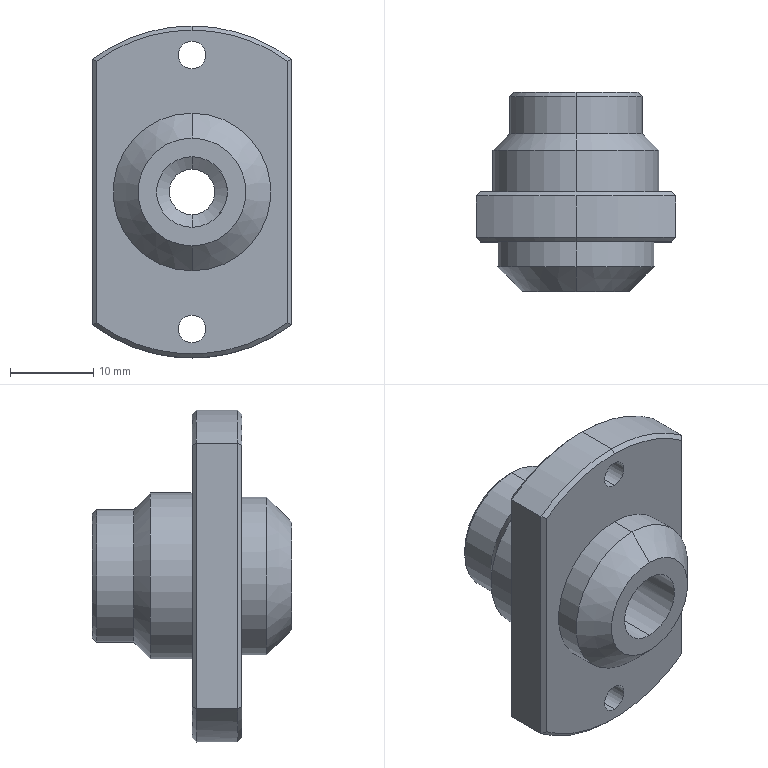Part | SolidWorks | features ICE 7, Chamfer 4, HoleWzd 4, Extrusion 1, RevCut 1 | 1 solid | 52 faces | box 24 x 24 x 40 mm | volume 8141 mm3 | cylinder 25 | cone 14 | plane 13 | commonest cylinder face diameters 3.3 x4 11 x4 40 x3 4.2 x2 5.5 x2 8.5 x2
STEP:
#1=CARTESIAN_POINT('',(0.,-5.,8.));
#2=VERTEX_POINT('',#1);
#3=CARTESIAN_POINT('',(0.,-5.,-8.));
#4=VERTEX_POINT('',#3);
#5=CARTESIAN_POINT('',(0.,-5.,0.));
#6=DIRECTION('',(0.,1.,0.));
#7=DIRECTION('',(0.,0.,1.));
#8=AXIS2_PLACEMENT_3D('',#5,#6,#7);
#9=CIRCLE('',#8,8.);
#10=EDGE_CURVE('',#2,#4,#9,.T.);
#11=ORIENTED_EDGE('',*,*,#10,.F.);
#12=CARTESIAN_POINT('',(0.,-7.,10.));
#13=VERTEX_POINT('',#12);
#14=CARTESIAN_POINT('',(0.,-7.,10.));
#15=DIRECTION('',(0.,-0.7071,0.7071));
#16=VECTOR('',#15,1000.);
#17=LINE('',#14,#16);
#18=EDGE_CURVE('',#2,#13,#17,.T.);
#19=ORIENTED_EDGE('',*,*,#18,.T.);
#20=CARTESIAN_POINT('',(0.,-7.,-10.));
#21=VERTEX_POINT('',#20);
#22=CARTESIAN_POINT('',(0.,-7.,0.));
#23=DIRECTION('',(0.,1.,0.));
#24=DIRECTION('',(0.,0.,1.));
#25=AXIS2_PLACEMENT_3D('',#22,#23,#24);
#26=CIRCLE('',#25,10.);
#27=EDGE_CURVE('',#13,#21,#26,.T.);
#28=ORIENTED_EDGE('',*,*,#27,.T.);
#29=CARTESIAN_POINT('',(0.,-7.,-10.));
#30=DIRECTION('',(0.,-0.7071,-0.7071));
#31=VECTOR('',#30,1000.);
#32=LINE('',#29,#31);
#33=EDGE_CURVE('',#4,#21,#32,.T.);
#34=ORIENTED_EDGE('',*,*,#33,.F.);
#35=EDGE_LOOP('',(#11,#19,#28,#34));
#36=FACE_OUTER_BOUND('',#35,.T.);
#37=CARTESIAN_POINT('',(0.,-7.,0.));
#38=DIRECTION('',(0.,-1.,0.));
#39=DIRECTION('',(0.,0.,-1.));
#40=AXIS2_PLACEMENT_3D('',#37,#38,#39);
#41=CONICAL_SURFACE('',#40,10.,0.7854);
#42=ADVANCED_FACE('',(#36),#41,.T.);
#43=ORIENTED_EDGE('',*,*,#27,.F.);
#44=CARTESIAN_POINT('',(0.,-12.,10.));
#45=VERTEX_POINT('',#44);
#46=CARTESIAN_POINT('',(0.,-7.,10.));
#47=DIRECTION('',(0.,-1.,0.));
#48=VECTOR('',#47,1000.);
#49=LINE('',#46,#48);
#50=EDGE_CURVE('',#13,#45,#49,.T.);
#51=ORIENTED_EDGE('',*,*,#50,.T.);
#52=CARTESIAN_POINT('',(0.,-12.,-10.));
#53=VERTEX_POINT('',#52);
#54=CARTESIAN_POINT('',(0.,-12.,0.));
#55=DIRECTION('',(0.,1.,0.));
#56=DIRECTION('',(0.,0.,-1.));
#57=AXIS2_PLACEMENT_3D('',#54,#55,#56);
#58=CIRCLE('',#57,10.);
#59=EDGE_CURVE('',#45,#53,#58,.T.);
#60=ORIENTED_EDGE('',*,*,#59,.T.);
#61=CARTESIAN_POINT('',(0.,-7.,-10.));
#62=DIRECTION('',(0.,-1.,0.));
#63=VECTOR('',#62,1000.);
#64=LINE('',#61,#63);
#65=EDGE_CURVE('',#21,#53,#64,.T.);
#66=ORIENTED_EDGE('',*,*,#65,.F.);
#67=EDGE_LOOP('',(#43,#51,#60,#66));
#68=FACE_OUTER_BOUND('',#67,.T.);
#69=CARTESIAN_POINT('',(0.,-7.,0.));
#70=DIRECTION('',(0.,-1.,0.));
#71=DIRECTION('',(0.,0.,-1.));
#72=AXIS2_PLACEMENT_3D('',#69,#70,#71);
#73=CYLINDRICAL_SURFACE('',#72,10.);
#74=ADVANCED_FACE('',(#68),#73,.T.);
#75=CARTESIAN_POINT('',(0.,-2.,5.75));
#76=VERTEX_POINT('',#75);
#77=CARTESIAN_POINT('',(0.,-2.,-5.75));
#78=VERTEX_POINT('',#77);
#79=CARTESIAN_POINT('',(0.,-2.,0.));
#80=DIRECTION('',(0.,-1.,0.));
#81=DIRECTION('',(0.,0.,-1.));
#82=AXIS2_PLACEMENT_3D('',#79,#80,#81);
#83=CIRCLE('',#82,5.75);
#84=EDGE_CURVE('',#76,#78,#83,.T.);
#85=ORIENTED_EDGE('',*,*,#84,.F.);
#86=CARTESIAN_POINT('',(0.,-3.,5.75));
#87=VERTEX_POINT('',#86);
#88=CARTESIAN_POINT('',(0.,-12.,5.75));
#89=DIRECTION('',(0.,-1.,0.));
#90=VECTOR('',#89,1000.);
#91=LINE('',#88,#90);
#92=EDGE_CURVE('',#76,#87,#91,.T.);
#93=ORIENTED_EDGE('',*,*,#92,.T.);
#94=CARTESIAN_POINT('',(0.,-3.,-5.75));
#95=VERTEX_POINT('',#94);
#96=CARTESIAN_POINT('',(0.,-3.,0.));
#97=DIRECTION('',(0.,-1.,0.));
#98=DIRECTION('',(0.,0.,-1.));
#99=AXIS2_PLACEMENT_3D('',#96,#97,#98);
#100=CIRCLE('',#99,5.75);
#101=EDGE_CURVE('',#87,#95,#100,.T.);
#102=ORIENTED_EDGE('',*,*,#101,.T.);
#103=CARTESIAN_POINT('',(0.,-12.,-5.75));
#104=DIRECTION('',(0.,-1.,0.));
#105=VECTOR('',#104,1000.);
#106=LINE('',#103,#105);
#107=EDGE_CURVE('',#78,#95,#106,.T.);
#108=ORIENTED_EDGE('',*,*,#107,.F.);
#109=EDGE_LOOP('',(#85,#93,#102,#108));
#110=FACE_OUTER_BOUND('',#109,.T.);
#111=CARTESIAN_POINT('',(0.,-12.,0.));
#112=DIRECTION('',(0.,-1.,0.));
#113=DIRECTION('',(0.,0.,-1.));
#114=AXIS2_PLACEMENT_3D('',#111,#112,#113);
#115=CYLINDRICAL_SURFACE('',#114,5.75);
#116=ADVANCED_FACE('',(#110),#115,.F.);
#117=CARTESIAN_POINT('',(0.,0.,7.5));
#118=VERTEX_POINT('',#117);
#119=CARTESIAN_POINT('',(0.,0.,-7.5));
#120=VERTEX_POINT('',#119);
#121=CARTESIAN_POINT('',(0.,0.,0.));
#122=DIRECTION('',(0.,1.,0.));
#123=DIRECTION('',(0.,0.,1.));
#124=AXIS2_PLACEMENT_3D('',#121,#122,#123);
#125=CIRCLE('',#124,7.5);
#126=EDGE_CURVE('',#118,#120,#125,.T.);
#127=ORIENTED_EDGE('',*,*,#126,.F.);
#128=CARTESIAN_POINT('',(0.,-0.5,8.));
#129=VERTEX_POINT('',#128);
#130=CARTESIAN_POINT('',(0.,0.,7.5));
#131=DIRECTION('',(0.,-0.7071,0.7071));
#132=VECTOR('',#131,1000.);
#133=LINE('',#130,#132);
#134=EDGE_CURVE('',#118,#129,#133,.T.);
#135=ORIENTED_EDGE('',*,*,#134,.T.);
#136=CARTESIAN_POINT('',(0.,-0.5,-8.));
#137=VERTEX_POINT('',#136);
#138=CARTESIAN_POINT('',(0.,-0.5,0.));
#139=DIRECTION('',(0.,-1.,0.));
#140=DIRECTION('',(0.,0.,1.));
#141=AXIS2_PLACEMENT_3D('',#138,#139,#140);
#142=CIRCLE('',#141,8.);
#143=EDGE_CURVE('',#137,#129,#142,.T.);
#144=ORIENTED_EDGE('',*,*,#143,.F.);
#145=CARTESIAN_POINT('',(0.,0.,-7.5));
#146=DIRECTION('',(0.,-0.7071,-0.7071));
#147=VECTOR('',#146,1000.);
#148=LINE('',#145,#147);
#149=EDGE_CURVE('',#120,#137,#148,.T.);
#150=ORIENTED_EDGE('',*,*,#149,.F.);
#151=EDGE_LOOP('',(#127,#135,#144,#150));
#152=FACE_OUTER_BOUND('',#151,.T.);
#153=CARTESIAN_POINT('',(0.,0.,0.));
#154=DIRECTION('',(0.,-1.,0.));
#155=DIRECTION('',(0.,0.,-1.));
#156=AXIS2_PLACEMENT_3D('',#153,#154,#155);
#157=CONICAL_SURFACE('',#156,7.5,0.7854);
#158=ADVANCED_FACE('',(#152),#157,.T.);
#159=CARTESIAN_POINT('',(0.,-12.,-19.5));
#160=VERTEX_POINT('',#159);
#161=CARTESIAN_POINT('',(-11.5,-12.,-15.748));
#162=VERTEX_POINT('',#161);
#163=CARTESIAN_POINT('',(0.,-12.,0.));
#164=DIRECTION('',(0.,1.,0.));
#165=DIRECTION('',(0.,0.,-1.));
#166=AXIS2_PLACEMENT_3D('',#163,#164,#165);
#167=CIRCLE('',#166,19.5);
#168=EDGE_CURVE('',#160,#162,#167,.T.);
#169=ORIENTED_EDGE('',*,*,#168,.F.);
#170=CARTESIAN_POINT('',(0.,-12.5,-20.));
#171=VERTEX_POINT('',#170);
#172=CARTESIAN_POINT('',(0.,-12.5,-20.));
#173=DIRECTION('',(0.,-0.7071,-0.7071));
#174=VECTOR('',#173,1000.);
#175=LINE('',#172,#174);
#176=EDGE_CURVE('',#160,#171,#175,.T.);
#177=ORIENTED_EDGE('',*,*,#176,.T.);
#178=CARTESIAN_POINT('',(-12.,-12.5,-16.));
#179=VERTEX_POINT('',#178);
#180=CARTESIAN_POINT('',(0.,-12.5,0.));
#181=DIRECTION('',(0.,-1.,0.));
#182=DIRECTION('',(0.,0.,-1.));
#183=AXIS2_PLACEMENT_3D('',#180,#181,#182);
#184=CIRCLE('',#183,20.);
#185=EDGE_CURVE('',#179,#171,#184,.T.);
#186=ORIENTED_EDGE('',*,*,#185,.F.);
#187=CARTESIAN_POINT('',(-11.5,-12.,-15.748));
#188=CARTESIAN_POINT('',(-11.667,-12.167,-15.833));
#189=CARTESIAN_POINT('',(-11.833,-12.333,-15.917));
#190=CARTESIAN_POINT('',(-12.,-12.5,-16.));
#191=B_SPLINE_CURVE_WITH_KNOTS('',3,(#187,#188,#189,#190),.UNSPECIFIED.,.F.,.F.,(4,4),(0.,0.0007507),.UNSPECIFIED.);
#192=EDGE_CURVE('',#162,#179,#191,.T.);
#193=ORIENTED_EDGE('',*,*,#192,.F.);
#194=EDGE_LOOP('',(#169,#177,#186,#193));
#195=FACE_OUTER_BOUND('',#194,.T.);
#196=CARTESIAN_POINT('',(0.,-12.5,0.));
#197=DIRECTION('',(0.,-1.,0.));
#198=DIRECTION('',(0.,0.,-1.));
#199=AXIS2_PLACEMENT_3D('',#196,#197,#198);
#200=CONICAL_SURFACE('',#199,20.,0.7854);
#201=ADVANCED_FACE('',(#195),#200,.T.);
#202=CARTESIAN_POINT('',(0.,-18.,19.5));
#203=VERTEX_POINT('',#202);
#204=CARTESIAN_POINT('',(-11.5,-18.,15.748));
#205=VERTEX_POINT('',#204);
#206=CARTESIAN_POINT('',(0.,-18.,0.));
#207=DIRECTION('',(0.,-1.,0.));
#208=DIRECTION('',(0.,0.,-1.));
#209=AXIS2_PLACEMENT_3D('',#206,#207,#208);
#210=CIRCLE('',#209,19.5);
#211=EDGE_CURVE('',#203,#205,#210,.T.);
#212=ORIENTED_EDGE('',*,*,#211,.F.);
#213=CARTESIAN_POINT('',(0.,-17.5,20.));
#214=VERTEX_POINT('',#213);
#215=CARTESIAN_POINT('',(0.,-18.,19.5));
#216=DIRECTION('',(0.,0.7071,0.7071));
#217=VECTOR('',#216,1000.);
#218=LINE('',#215,#217);
#219=EDGE_CURVE('',#203,#214,#218,.T.);
#220=ORIENTED_EDGE('',*,*,#219,.T.);
#221=CARTESIAN_POINT('',(-12.,-17.5,16.));
#222=VERTEX_POINT('',#221);
#223=CARTESIAN_POINT('',(0.,-17.5,0.));
#224=DIRECTION('',(0.,1.,0.));
#225=DIRECTION('',(0.,0.,-1.));
#226=AXIS2_PLACEMENT_3D('',#223,#224,#225);
#227=CIRCLE('',#226,20.);
#228=EDGE_CURVE('',#222,#214,#227,.T.);
#229=ORIENTED_EDGE('',*,*,#228,.F.);
#230=CARTESIAN_POINT('',(-11.5,-18.,15.748));
#231=CARTESIAN_POINT('',(-11.667,-17.833,15.833));
#232=CARTESIAN_POINT('',(-11.833,-17.667,15.917));
#233=CARTESIAN_POINT('',(-12.,-17.5,16.));
#234=B_SPLINE_CURVE_WITH_KNOTS('',3,(#230,#231,#232,#233),.UNSPECIFIED.,.F.,.F.,(4,4),(0.,0.0007507),.UNSPECIFIED.);
#235=EDGE_CURVE('',#205,#222,#234,.T.);
#236=ORIENTED_EDGE('',*,*,#235,.F.);
#237=EDGE_LOOP('',(#212,#220,#229,#236));
#238=FACE_OUTER_BOUND('',#237,.T.);
#239=CARTESIAN_POINT('',(0.,-18.,0.));
#240=DIRECTION('',(0.,1.,0.));
#241=DIRECTION('',(0.,0.,1.));
#242=AXIS2_PLACEMENT_3D('',#239,#240,#241);
#243=CONICAL_SURFACE('',#242,19.5,0.7854);
#244=ADVANCED_FACE('',(#238),#243,.T.);
#245=CARTESIAN_POINT('',(3.695,-15.,2.1));
#246=VERTEX_POINT('',#245);
#247=CARTESIAN_POINT('',(3.695,-15.,-2.1));
#248=VERTEX_POINT('',#247);
#249=CARTESIAN_POINT('',(3.695,-15.,2.1));
#250=CARTESIAN_POINT('',(3.695,-15.139,2.1));
#251=CARTESIAN_POINT('',(3.703,-15.281,2.086));
#252=CARTESIAN_POINT('',(3.734,-15.552,2.031));
#253=CARTESIAN_POINT('',(3.756,-15.684,1.99));
#254=CARTESIAN_POINT('',(3.81,-15.939,1.883));
#255=CARTESIAN_POINT('',(3.842,-16.059,1.819));
#256=CARTESIAN_POINT('',(3.91,-16.284,1.668));
#257=CARTESIAN_POINT('',(3.947,-16.389,1.58));
#258=CARTESIAN_POINT('',(4.018,-16.58,1.39));
#259=CARTESIAN_POINT('',(4.053,-16.666,1.286));
#260=CARTESIAN_POINT('',(4.117,-16.818,1.06));
#261=CARTESIAN_POINT('',(4.147,-16.884,0.938));
#262=CARTESIAN_POINT('',(4.196,-16.99,0.686));
#263=CARTESIAN_POINT('',(4.216,-17.03,0.5547));
#264=CARTESIAN_POINT('',(4.243,-17.086,0.2804));
#265=CARTESIAN_POINT('',(4.25,-17.1,0.1406));
#266=CARTESIAN_POINT('',(4.25,-17.1,-0.1373));
#267=CARTESIAN_POINT('',(4.243,-17.086,-0.2781));
#268=CARTESIAN_POINT('',(4.216,-17.031,-0.5516));
#269=CARTESIAN_POINT('',(4.197,-16.99,-0.6835));
#270=CARTESIAN_POINT('',(4.123,-16.831,-1.065));
#271=CARTESIAN_POINT('',(4.053,-16.676,-1.294));
#272=CARTESIAN_POINT('',(3.946,-16.388,-1.582));
#273=CARTESIAN_POINT('',(3.91,-16.284,-1.667));
#274=CARTESIAN_POINT('',(3.842,-16.059,-1.818));
#275=CARTESIAN_POINT('',(3.81,-15.938,-1.884));
#276=CARTESIAN_POINT('',(3.756,-15.685,-1.99));
#277=CARTESIAN_POINT('',(3.734,-15.555,-2.03));
#278=CARTESIAN_POINT('',(3.703,-15.283,-2.085));
#279=CARTESIAN_POINT('',(3.695,-15.141,-2.1));
#280=CARTESIAN_POINT('',(3.695,-15.,-2.1));
#281=B_SPLINE_CURVE_WITH_KNOTS('',3,(#249,#250,#251,#252,#253,#254,#255,#256,#257,#258,#259,#260,#261,#262,#263,#264,#265,#266,#267,#268,#269,#270,#271,#272,#273,#274,#275,#276,#277,#278,#279,#280),.UNSPECIFIED.,.F.,.F.,(4,2,2,2,2,2,2,2,2,2,2,2,2,2,2,4),(0.006676,0.007093,0.007509,0.007926,0.008343,0.008759,0.009176,0.009592,0.01001,0.01043,0.01084,0.01168,0.01209,0.01251,0.01292,0.01334),.UNSPECIFIED.);
#282=EDGE_CURVE('',#246,#248,#281,.T.);
#283=ORIENTED_EDGE('',*,*,#282,.F.);
#284=CARTESIAN_POINT('',(12.,-15.,2.1));
#285=VERTEX_POINT('',#284);
#286=CARTESIAN_POINT('',(12.,-15.,2.1));
#287=DIRECTION('',(1.,0.,0.));
#288=VECTOR('',#287,1000.);
#289=LINE('',#286,#288);
#290=EDGE_CURVE('',#246,#285,#289,.T.);
#291=ORIENTED_EDGE('',*,*,#290,.T.);
#292=CARTESIAN_POINT('',(12.,-15.,-2.1));
#293=VERTEX_POINT('',#292);
#294=CARTESIAN_POINT('',(12.,-15.,0.));
#295=DIRECTION('',(1.,0.,0.));
#296=DIRECTION('',(0.,0.,-1.));
#297=AXIS2_PLACEMENT_3D('',#294,#295,#296);
#298=CIRCLE('',#297,2.1);
#299=EDGE_CURVE('',#285,#293,#298,.T.);
#300=ORIENTED_EDGE('',*,*,#299,.T.);
#301=CARTESIAN_POINT('',(12.,-15.,-2.1));
#302=DIRECTION('',(1.,0.,0.));
#303=VECTOR('',#302,1000.);
#304=LINE('',#301,#303);
#305=EDGE_CURVE('',#248,#293,#304,.T.);
#306=ORIENTED_EDGE('',*,*,#305,.F.);
#307=EDGE_LOOP('',(#283,#291,#300,#306));
#308=FACE_OUTER_BOUND('',#307,.T.);
#309=CARTESIAN_POINT('',(12.,-15.,0.));
#310=DIRECTION('',(1.,0.,0.));
#311=DIRECTION('',(0.,0.,-1.));
#312=AXIS2_PLACEMENT_3D('',#309,#310,#311);
#313=CYLINDRICAL_SURFACE('',#312,2.1);
#314=ADVANCED_FACE('',(#308),#313,.F.);
#315=CARTESIAN_POINT('',(0.,-10.,4.25));
#316=VERTEX_POINT('',#315);
#317=CARTESIAN_POINT('',(0.,-10.,-4.25));
#318=VERTEX_POINT('',#317);
#319=CARTESIAN_POINT('',(0.,-10.,0.));
#320=DIRECTION('',(0.,-1.,0.));
#321=DIRECTION('',(0.,0.,-1.));
#322=AXIS2_PLACEMENT_3D('',#319,#320,#321);
#323=CIRCLE('',#322,4.25);
#324=EDGE_CURVE('',#316,#318,#323,.T.);
#325=ORIENTED_EDGE('',*,*,#324,.F.);
#326=CARTESIAN_POINT('',(0.,-24.,4.25));
#327=VERTEX_POINT('',#326);
#328=CARTESIAN_POINT('',(0.,-24.,4.25));
#329=DIRECTION('',(0.,-1.,0.));
#330=VECTOR('',#329,1000.);
#331=LINE('',#328,#330);
#332=EDGE_CURVE('',#316,#327,#331,.T.);
#333=ORIENTED_EDGE('',*,*,#332,.T.);
#334=CARTESIAN_POINT('',(0.,-24.,-4.25));
#335=VERTEX_POINT('',#334);
#336=CARTESIAN_POINT('',(0.,-24.,0.));
#337=DIRECTION('',(0.,-1.,0.));
#338=DIRECTION('',(0.,0.,-1.));
#339=AXIS2_PLACEMENT_3D('',#336,#337,#338);
#340=CIRCLE('',#339,4.25);
#341=EDGE_CURVE('',#327,#335,#340,.T.);
#342=ORIENTED_EDGE('',*,*,#341,.T.);
#343=CARTESIAN_POINT('',(0.,-24.,-4.25));
#344=DIRECTION('',(0.,-1.,0.));
#345=VECTOR('',#344,1000.);
#346=LINE('',#343,#345);
#347=EDGE_CURVE('',#318,#335,#346,.T.);
#348=ORIENTED_EDGE('',*,*,#347,.F.);
#349=EDGE_LOOP('',(#325,#333,#342,#348));
#350=FACE_OUTER_BOUND('',#349,.T.);
#351=CARTESIAN_POINT('',(0.,-24.,0.));
#352=DIRECTION('',(0.,-1.,0.));
#353=DIRECTION('',(0.,0.,-1.));
#354=AXIS2_PLACEMENT_3D('',#351,#352,#353);
#355=CYLINDRICAL_SURFACE('',#354,4.25);
#356=ADVANCED_FACE('',(#350),#355,.F.);
#357=CARTESIAN_POINT('',(0.,-9.099,2.75));
#358=VERTEX_POINT('',#357);
#359=CARTESIAN_POINT('',(0.,-9.099,-2.75));
#360=VERTEX_POINT('',#359);
#361=CARTESIAN_POINT('',(0.,-9.099,0.));
#362=DIRECTION('',(0.,-1.,0.));
#363=DIRECTION('',(0.,0.,-1.));
#364=AXIS2_PLACEMENT_3D('',#361,#362,#363);
#365=CIRCLE('',#364,2.75);
#366=EDGE_CURVE('',#358,#360,#365,.T.);
#367=ORIENTED_EDGE('',*,*,#366,.F.);
#368=CARTESIAN_POINT('',(0.,-10.,4.25));
#369=DIRECTION('',(0.,-0.515,0.8572));
#370=VECTOR('',#369,1000.);
#371=LINE('',#368,#370);
#372=EDGE_CURVE('',#358,#316,#371,.T.);
#373=ORIENTED_EDGE('',*,*,#372,.T.);
#374=ORIENTED_EDGE('',*,*,#324,.T.);
#375=CARTESIAN_POINT('',(0.,-10.,-4.25));
#376=DIRECTION('',(0.,-0.515,-0.8572));
#377=VECTOR('',#376,1000.);
#378=LINE('',#375,#377);
#379=EDGE_CURVE('',#360,#318,#378,.T.);
#380=ORIENTED_EDGE('',*,*,#379,.F.);
#381=EDGE_LOOP('',(#367,#373,#374,#380));
#382=FACE_OUTER_BOUND('',#381,.T.);
#383=CARTESIAN_POINT('',(0.,-10.,0.));
#384=DIRECTION('',(0.,-1.,0.));
#385=DIRECTION('',(0.,0.,-1.));
#386=AXIS2_PLACEMENT_3D('',#383,#384,#385);
#387=CONICAL_SURFACE('',#386,4.25,1.03);
#388=ADVANCED_FACE('',(#382),#387,.F.);
#389=ORIENTED_EDGE('',*,*,#366,.T.);
#390=CARTESIAN_POINT('',(0.,-7.,-2.75));
#391=VERTEX_POINT('',#390);
#392=CARTESIAN_POINT('',(0.,-7.,-2.75));
#393=DIRECTION('',(0.,1.,0.));
#394=VECTOR('',#393,1000.);
#395=LINE('',#392,#394);
#396=EDGE_CURVE('',#360,#391,#395,.T.);
#397=ORIENTED_EDGE('',*,*,#396,.T.);
#398=CARTESIAN_POINT('',(0.,-7.,2.75));
#399=VERTEX_POINT('',#398);
#400=CARTESIAN_POINT('',(0.,-7.,0.));
#401=DIRECTION('',(0.,1.,0.));
#402=DIRECTION('',(0.,0.,1.));
#403=AXIS2_PLACEMENT_3D('',#400,#401,#402);
#404=CIRCLE('',#403,2.75);
#405=EDGE_CURVE('',#391,#399,#404,.T.);
#406=ORIENTED_EDGE('',*,*,#405,.T.);
#407=CARTESIAN_POINT('',(0.,-7.,2.75));
#408=DIRECTION('',(0.,1.,0.));
#409=VECTOR('',#408,1000.);
#410=LINE('',#407,#409);
#411=EDGE_CURVE('',#358,#399,#410,.T.);
#412=ORIENTED_EDGE('',*,*,#411,.F.);
#413=EDGE_LOOP('',(#389,#397,#406,#412));
#414=FACE_OUTER_BOUND('',#413,.T.);
#415=CARTESIAN_POINT('',(0.,-7.,0.));
#416=DIRECTION('',(0.,1.,0.));
#417=DIRECTION('',(0.,0.,1.));
#418=AXIS2_PLACEMENT_3D('',#415,#416,#417);
#419=CYLINDRICAL_SURFACE('',#418,2.75);
#420=ADVANCED_FACE('',(#414),#419,.F.);
#421=CARTESIAN_POINT('',(0.,-7.,-5.5));
#422=VERTEX_POINT('',#421);
#423=CARTESIAN_POINT('',(0.,-7.,5.5));
#424=VERTEX_POINT('',#423);
#425=CARTESIAN_POINT('',(0.,-7.,0.));
#426=DIRECTION('',(0.,1.,0.));
#427=DIRECTION('',(0.,0.,1.));
#428=AXIS2_PLACEMENT_3D('',#425,#426,#427);
#429=CIRCLE('',#428,5.5);
#430=EDGE_CURVE('',#422,#424,#429,.T.);
#431=ORIENTED_EDGE('',*,*,#430,.F.);
#432=CARTESIAN_POINT('',(0.,-3.,-5.5));
#433=VERTEX_POINT('',#432);
#434=CARTESIAN_POINT('',(0.,-7.,-5.5));
#435=DIRECTION('',(0.,1.,0.));
#436=VECTOR('',#435,1000.);
#437=LINE('',#434,#436);
#438=EDGE_CURVE('',#422,#433,#437,.T.);
#439=ORIENTED_EDGE('',*,*,#438,.T.);
#440=CARTESIAN_POINT('',(0.,-3.,5.5));
#441=VERTEX_POINT('',#440);
#442=CARTESIAN_POINT('',(0.,-3.,0.));
#443=DIRECTION('',(0.,1.,0.));
#444=DIRECTION('',(0.,0.,-1.));
#445=AXIS2_PLACEMENT_3D('',#442,#443,#444);
#446=CIRCLE('',#445,5.5);
#447=EDGE_CURVE('',#433,#441,#446,.T.);
#448=ORIENTED_EDGE('',*,*,#447,.T.);
#449=CARTESIAN_POINT('',(0.,-7.,5.5));
#450=DIRECTION('',(0.,1.,0.));
#451=VECTOR('',#450,1000.);
#452=LINE('',#449,#451);
#453=EDGE_CURVE('',#424,#441,#452,.T.);
#454=ORIENTED_EDGE('',*,*,#453,.F.);
#455=EDGE_LOOP('',(#431,#439,#448,#454));
#456=FACE_OUTER_BOUND('',#455,.T.);
#457=CARTESIAN_POINT('',(0.,-7.,0.));
#458=DIRECTION('',(0.,1.,0.));
#459=DIRECTION('',(0.,0.,1.));
#460=AXIS2_PLACEMENT_3D('',#457,#458,#459);
#461=CYLINDRICAL_SURFACE('',#460,5.5);
#462=ADVANCED_FACE('',(#456),#461,.F.);
#463=CARTESIAN_POINT('',(0.,-24.,-6.5));
#464=VERTEX_POINT('',#463);
#465=CARTESIAN_POINT('',(0.,-24.,6.5));
#466=VERTEX_POINT('',#465);
#467=CARTESIAN_POINT('',(0.,-24.,0.));
#468=DIRECTION('',(0.,-1.,0.));
#469=DIRECTION('',(0.,0.,-1.));
#470=AXIS2_PLACEMENT_3D('',#467,#468,#469);
#471=CIRCLE('',#470,6.5);
#472=EDGE_CURVE('',#464,#466,#471,.T.);
#473=ORIENTED_EDGE('',*,*,#472,.F.);
#474=CARTESIAN_POINT('',(0.,-21.,-9.5));
#475=VERTEX_POINT('',#474);
#476=CARTESIAN_POINT('',(0.,-24.,-6.5));
#477=DIRECTION('',(0.,0.7071,-0.7071));
#478=VECTOR('',#477,1000.);
#479=LINE('',#476,#478);
#480=EDGE_CURVE('',#464,#475,#479,.T.);
#481=ORIENTED_EDGE('',*,*,#480,.T.);
#482=CARTESIAN_POINT('',(0.,-21.,9.5));
#483=VERTEX_POINT('',#482);
#484=CARTESIAN_POINT('',(0.,-21.,0.));
#485=DIRECTION('',(0.,1.,0.));
#486=DIRECTION('',(0.,0.,-1.));
#487=AXIS2_PLACEMENT_3D('',#484,#485,#486);
#488=CIRCLE('',#487,9.5);
#489=EDGE_CURVE('',#483,#475,#488,.T.);
#490=ORIENTED_EDGE('',*,*,#489,.F.);
#491=CARTESIAN_POINT('',(0.,-24.,6.5));
#492=DIRECTION('',(0.,0.7071,0.7071));
#493=VECTOR('',#492,1000.);
#494=LINE('',#491,#493);
#495=EDGE_CURVE('',#466,#483,#494,.T.);
#496=ORIENTED_EDGE('',*,*,#495,.F.);
#497=EDGE_LOOP('',(#473,#481,#490,#496));
#498=FACE_OUTER_BOUND('',#497,.T.);
#499=CARTESIAN_POINT('',(0.,-24.,0.));
#500=DIRECTION('',(0.,1.,0.));
#501=DIRECTION('',(0.,0.,1.));
#502=AXIS2_PLACEMENT_3D('',#499,#500,#501);
#503=CONICAL_SURFACE('',#502,6.5,0.7854);
#504=ADVANCED_FACE('',(#498),#503,.T.);
#505=CARTESIAN_POINT('',(0.,-18.,-14.85));
#506=VERTEX_POINT('',#505);
#507=CARTESIAN_POINT('',(0.,-18.,-18.15));
#508=VERTEX_POINT('',#507);
#509=CARTESIAN_POINT('',(0.,-18.,-16.5));
#510=DIRECTION('',(0.,-1.,0.));
#511=DIRECTION('',(0.,0.,-1.));
#512=AXIS2_PLACEMENT_3D('',#509,#510,#511);
#513=CIRCLE('',#512,1.65);
#514=EDGE_CURVE('',#506,#508,#513,.T.);
#515=ORIENTED_EDGE('',*,*,#514,.T.);
#516=CARTESIAN_POINT('',(0.,-12.,-18.15));
#517=VERTEX_POINT('',#516);
#518=CARTESIAN_POINT('',(0.,-12.,-18.15));
#519=DIRECTION('',(0.,1.,0.));
#520=VECTOR('',#519,1000.);
#521=LINE('',#518,#520);
#522=EDGE_CURVE('',#508,#517,#521,.T.);
#523=ORIENTED_EDGE('',*,*,#522,.T.);
#524=CARTESIAN_POINT('',(0.,-12.,-14.85));
#525=VERTEX_POINT('',#524);
#526=CARTESIAN_POINT('',(0.,-12.,-16.5));
#527=DIRECTION('',(0.,1.,0.));
#528=DIRECTION('',(0.,0.,1.));
#529=AXIS2_PLACEMENT_3D('',#526,#527,#528);
#530=CIRCLE('',#529,1.65);
#531=EDGE_CURVE('',#517,#525,#530,.T.);
#532=ORIENTED_EDGE('',*,*,#531,.T.);
#533=CARTESIAN_POINT('',(0.,-12.,-14.85));
#534=DIRECTION('',(0.,1.,0.));
#535=VECTOR('',#534,1000.);
#536=LINE('',#533,#535);
#537=EDGE_CURVE('',#506,#525,#536,.T.);
#538=ORIENTED_EDGE('',*,*,#537,.F.);
#539=EDGE_LOOP('',(#515,#523,#532,#538));
#540=FACE_OUTER_BOUND('',#539,.T.);
#541=CARTESIAN_POINT('',(0.,-12.,-16.5));
#542=DIRECTION('',(0.,1.,0.));
#543=DIRECTION('',(0.,0.,1.));
#544=AXIS2_PLACEMENT_3D('',#541,#542,#543);
#545=CYLINDRICAL_SURFACE('',#544,1.65);
#546=ADVANCED_FACE('',(#540),#545,.F.);
#547=CARTESIAN_POINT('',(0.,-18.,18.15));
#548=VERTEX_POINT('',#547);
#549=CARTESIAN_POINT('',(0.,-18.,14.85));
#550=VERTEX_POINT('',#549);
#551=CARTESIAN_POINT('',(0.,-18.,16.5));
#552=DIRECTION('',(0.,-1.,0.));
#553=DIRECTION('',(0.,0.,-1.));
#554=AXIS2_PLACEMENT_3D('',#551,#552,#553);
#555=CIRCLE('',#554,1.65);
#556=EDGE_CURVE('',#548,#550,#555,.T.);
#557=ORIENTED_EDGE('',*,*,#556,.T.);
#558=CARTESIAN_POINT('',(0.,-12.,14.85));
#559=VERTEX_POINT('',#558);
#560=CARTESIAN_POINT('',(0.,-12.,14.85));
#561=DIRECTION('',(0.,1.,0.));
#562=VECTOR('',#561,1000.);
#563=LINE('',#560,#562);
#564=EDGE_CURVE('',#550,#559,#563,.T.);
#565=ORIENTED_EDGE('',*,*,#564,.T.);
#566=CARTESIAN_POINT('',(0.,-12.,18.15));
#567=VERTEX_POINT('',#566);
#568=CARTESIAN_POINT('',(0.,-12.,16.5));
#569=DIRECTION('',(0.,1.,0.));
#570=DIRECTION('',(0.,0.,1.));
#571=AXIS2_PLACEMENT_3D('',#568,#569,#570);
#572=CIRCLE('',#571,1.65);
#573=EDGE_CURVE('',#559,#567,#572,.T.);
#574=ORIENTED_EDGE('',*,*,#573,.T.);
#575=CARTESIAN_POINT('',(0.,-12.,18.15));
#576=DIRECTION('',(0.,1.,0.));
#577=VECTOR('',#576,1000.);
#578=LINE('',#575,#577);
#579=EDGE_CURVE('',#548,#567,#578,.T.);
#580=ORIENTED_EDGE('',*,*,#579,.F.);
#581=EDGE_LOOP('',(#557,#565,#574,#580));
#582=FACE_OUTER_BOUND('',#581,.T.);
#583=CARTESIAN_POINT('',(0.,-12.,16.5));
#584=DIRECTION('',(0.,1.,0.));
#585=DIRECTION('',(0.,0.,1.));
#586=AXIS2_PLACEMENT_3D('',#583,#584,#585);
#587=CYLINDRICAL_SURFACE('',#586,1.65);
#588=ADVANCED_FACE('',(#582),#587,.F.);
#589=ORIENTED_EDGE('',*,*,#489,.T.);
#590=CARTESIAN_POINT('',(0.,-18.,-9.5));
#591=VERTEX_POINT('',#590);
#592=CARTESIAN_POINT('',(0.,-24.,-9.5));
#593=DIRECTION('',(0.,1.,0.));
#594=VECTOR('',#593,1000.);
#595=LINE('',#592,#594);
#596=EDGE_CURVE('',#475,#591,#595,.T.);
#597=ORIENTED_EDGE('',*,*,#596,.T.);
#598=CARTESIAN_POINT('',(0.,-18.,9.5));
#599=VERTEX_POINT('',#598);
#600=CARTESIAN_POINT('',(0.,-18.,0.));
#601=DIRECTION('',(0.,-1.,0.));
#602=DIRECTION('',(0.,0.,-1.));
#603=AXIS2_PLACEMENT_3D('',#600,#601,#602);
#604=CIRCLE('',#603,9.5);
#605=EDGE_CURVE('',#591,#599,#604,.T.);
#606=ORIENTED_EDGE('',*,*,#605,.T.);
#607=CARTESIAN_POINT('',(0.,-24.,9.5));
#608=DIRECTION('',(0.,1.,0.));
#609=VECTOR('',#608,1000.);
#610=LINE('',#607,#609);
#611=EDGE_CURVE('',#483,#599,#610,.T.);
#612=ORIENTED_EDGE('',*,*,#611,.F.);
#613=EDGE_LOOP('',(#589,#597,#606,#612));
#614=FACE_OUTER_BOUND('',#613,.T.);
#615=CARTESIAN_POINT('',(0.,-24.,0.));
#616=DIRECTION('',(0.,1.,0.));
#617=DIRECTION('',(0.,0.,1.));
#618=AXIS2_PLACEMENT_3D('',#615,#616,#617);
#619=CYLINDRICAL_SURFACE('',#618,9.5);
#620=ADVANCED_FACE('',(#614),#619,.T.);
#621=ORIENTED_EDGE('',*,*,#228,.T.);
#622=CARTESIAN_POINT('',(0.,-12.5,20.));
#623=VERTEX_POINT('',#622);
#624=CARTESIAN_POINT('',(0.,-18.,20.));
#625=DIRECTION('',(0.,1.,0.));
#626=VECTOR('',#625,1000.);
#627=LINE('',#624,#626);
#628=EDGE_CURVE('',#214,#623,#627,.T.);
#629=ORIENTED_EDGE('',*,*,#628,.T.);
#630=CARTESIAN_POINT('',(-12.,-12.5,16.));
#631=VERTEX_POINT('',#630);
#632=CARTESIAN_POINT('',(0.,-12.5,0.));
#633=DIRECTION('',(0.,-1.,0.));
#634=DIRECTION('',(0.,0.,-1.));
#635=AXIS2_PLACEMENT_3D('',#632,#633,#634);
#636=CIRCLE('',#635,20.);
#637=EDGE_CURVE('',#623,#631,#636,.T.);
#638=ORIENTED_EDGE('',*,*,#637,.T.);
#639=CARTESIAN_POINT('',(-12.,-18.,16.));
#640=DIRECTION('',(0.,-1.,0.));
#641=VECTOR('',#640,1000.);
#642=LINE('',#639,#641);
#643=EDGE_CURVE('',#631,#222,#642,.T.);
#644=ORIENTED_EDGE('',*,*,#643,.T.);
#645=EDGE_LOOP('',(#621,#629,#638,#644));
#646=FACE_OUTER_BOUND('',#645,.T.);
#647=CARTESIAN_POINT('',(0.,-18.,0.));
#648=DIRECTION('',(0.,1.,0.));
#649=DIRECTION('',(0.,0.,1.));
#650=AXIS2_PLACEMENT_3D('',#647,#648,#649);
#651=CYLINDRICAL_SURFACE('',#650,20.);
#652=ADVANCED_FACE('',(#646),#651,.T.);
#653=ORIENTED_EDGE('',*,*,#10,.T.);
#654=CARTESIAN_POINT('',(0.,-12.,-8.));
#655=DIRECTION('',(0.,1.,0.));
#656=VECTOR('',#655,1000.);
#657=LINE('',#654,#656);
#658=EDGE_CURVE('',#4,#137,#657,.T.);
#659=ORIENTED_EDGE('',*,*,#658,.T.);
#660=ORIENTED_EDGE('',*,*,#143,.T.);
#661=CARTESIAN_POINT('',(0.,-12.,8.));
#662=DIRECTION('',(0.,1.,0.));
#663=VECTOR('',#662,1000.);
#664=LINE('',#661,#663);
#665=EDGE_CURVE('',#2,#129,#664,.T.);
#666=ORIENTED_EDGE('',*,*,#665,.F.);
#667=EDGE_LOOP('',(#653,#659,#660,#666));
#668=FACE_OUTER_BOUND('',#667,.T.);
#669=CARTESIAN_POINT('',(0.,-12.,0.));
#670=DIRECTION('',(0.,1.,0.));
#671=DIRECTION('',(0.,0.,1.));
#672=AXIS2_PLACEMENT_3D('',#669,#670,#671);
#673=CYLINDRICAL_SURFACE('',#672,8.);
#674=ADVANCED_FACE('',(#668),#673,.T.);
#675=CARTESIAN_POINT('',(0.,-2.,5.5));
#676=VERTEX_POINT('',#675);
#677=CARTESIAN_POINT('',(0.,-2.,-5.5));
#678=VERTEX_POINT('',#677);
#679=CARTESIAN_POINT('',(0.,-2.,0.));
#680=DIRECTION('',(0.,-1.,0.));
#681=DIRECTION('',(0.,0.,1.));
#682=AXIS2_PLACEMENT_3D('',#679,#680,#681);
#683=CIRCLE('',#682,5.5);
#684=EDGE_CURVE('',#676,#678,#683,.T.);
#685=ORIENTED_EDGE('',*,*,#684,.T.);
#686=CARTESIAN_POINT('',(0.,0.,-5.5));
#687=VERTEX_POINT('',#686);
#688=CARTESIAN_POINT('',(0.,-7.,-5.5));
#689=DIRECTION('',(0.,1.,0.));
#690=VECTOR('',#689,1000.);
#691=LINE('',#688,#690);
#692=EDGE_CURVE('',#678,#687,#691,.T.);
#693=ORIENTED_EDGE('',*,*,#692,.T.);
#694=CARTESIAN_POINT('',(0.,0.,5.5));
#695=VERTEX_POINT('',#694);
#696=CARTESIAN_POINT('',(0.,0.,0.));
#697=DIRECTION('',(0.,1.,0.));
#698=DIRECTION('',(0.,0.,1.));
#699=AXIS2_PLACEMENT_3D('',#696,#697,#698);
#700=CIRCLE('',#699,5.5);
#701=EDGE_CURVE('',#687,#695,#700,.T.);
#702=ORIENTED_EDGE('',*,*,#701,.T.);
#703=CARTESIAN_POINT('',(0.,-7.,5.5));
#704=DIRECTION('',(0.,1.,0.));
#705=VECTOR('',#704,1000.);
#706=LINE('',#703,#705);
#707=EDGE_CURVE('',#676,#695,#706,.T.);
#708=ORIENTED_EDGE('',*,*,#707,.F.);
#709=EDGE_LOOP('',(#685,#693,#702,#708));
#710=FACE_OUTER_BOUND('',#709,.T.);
#711=CARTESIAN_POINT('',(0.,-7.,0.));
#712=DIRECTION('',(0.,1.,0.));
#713=DIRECTION('',(0.,0.,1.));
#714=AXIS2_PLACEMENT_3D('',#711,#712,#713);
#715=CYLINDRICAL_SURFACE('',#714,5.5);
#716=ADVANCED_FACE('',(#710),#715,.F.);
#717=CARTESIAN_POINT('',(0.,-12.,16.5));
#718=DIRECTION('',(0.,1.,0.));
#719=DIRECTION('',(0.,0.,1.));
#720=AXIS2_PLACEMENT_3D('',#717,#718,#719);
#721=CIRCLE('',#720,1.65);
#722=EDGE_CURVE('',#567,#559,#721,.T.);
#723=ORIENTED_EDGE('',*,*,#722,.F.);
#724=ORIENTED_EDGE('',*,*,#573,.F.);
#725=EDGE_LOOP('',(#723,#724));
#726=FACE_BOUND('',#725,.T.);
#727=CARTESIAN_POINT('',(0.,-12.,-16.5));
#728=DIRECTION('',(0.,1.,0.));
#729=DIRECTION('',(0.,0.,1.));
#730=AXIS2_PLACEMENT_3D('',#727,#728,#729);
#731=CIRCLE('',#730,1.65);
#732=EDGE_CURVE('',#525,#517,#731,.T.);
#733=ORIENTED_EDGE('',*,*,#732,.F.);
#734=ORIENTED_EDGE('',*,*,#531,.F.);
#735=EDGE_LOOP('',(#733,#734));
#736=FACE_BOUND('',#735,.T.);
#737=CARTESIAN_POINT('',(11.5,-12.,-15.748));
#738=VERTEX_POINT('',#737);
#739=CARTESIAN_POINT('',(0.,-12.,0.));
#740=DIRECTION('',(0.,1.,0.));
#741=DIRECTION('',(0.,0.,-1.));
#742=AXIS2_PLACEMENT_3D('',#739,#740,#741);
#743=CIRCLE('',#742,19.5);
#744=EDGE_CURVE('',#738,#160,#743,.T.);
#745=ORIENTED_EDGE('',*,*,#744,.T.);
#746=ORIENTED_EDGE('',*,*,#168,.T.);
#747=CARTESIAN_POINT('',(-11.5,-12.,15.748));
#748=VERTEX_POINT('',#747);
#749=CARTESIAN_POINT('',(-11.5,-12.,0.));
#750=DIRECTION('',(0.,0.,1.));
#751=VECTOR('',#750,1000.);
#752=LINE('',#749,#751);
#753=EDGE_CURVE('',#162,#748,#752,.T.);
#754=ORIENTED_EDGE('',*,*,#753,.T.);
#755=CARTESIAN_POINT('',(11.5,-12.,15.748));
#756=VERTEX_POINT('',#755);
#757=CARTESIAN_POINT('',(0.,-12.,0.));
#758=DIRECTION('',(0.,1.,0.));
#759=DIRECTION('',(0.,0.,-1.));
#760=AXIS2_PLACEMENT_3D('',#757,#758,#759);
#761=CIRCLE('',#760,19.5);
#762=EDGE_CURVE('',#748,#756,#761,.T.);
#763=ORIENTED_EDGE('',*,*,#762,.T.);
#764=CARTESIAN_POINT('',(11.5,-12.,0.));
#765=DIRECTION('',(0.,0.,-1.));
#766=VECTOR('',#765,1000.);
#767=LINE('',#764,#766);
#768=EDGE_CURVE('',#756,#738,#767,.T.);
#769=ORIENTED_EDGE('',*,*,#768,.T.);
#770=EDGE_LOOP('',(#745,#746,#754,#763,#769));
#771=FACE_OUTER_BOUND('',#770,.T.);
#772=CARTESIAN_POINT('',(0.,-12.,0.));
#773=DIRECTION('',(0.,1.,0.));
#774=DIRECTION('',(0.,0.,-1.));
#775=AXIS2_PLACEMENT_3D('',#772,#773,#774);
#776=CIRCLE('',#775,10.);
#777=EDGE_CURVE('',#53,#45,#776,.T.);
#778=ORIENTED_EDGE('',*,*,#777,.F.);
#779=ORIENTED_EDGE('',*,*,#59,.F.);
#780=EDGE_LOOP('',(#778,#779));
#781=FACE_BOUND('',#780,.T.);
#782=CARTESIAN_POINT('',(0.,-12.,0.));
#783=DIRECTION('',(0.,-1.,0.));
#784=DIRECTION('',(0.,0.,-1.));
#785=AXIS2_PLACEMENT_3D('',#782,#783,#784);
#786=PLANE('',#785);
#787=ADVANCED_FACE('',(#726,#736,#771,#781),#786,.F.);
#788=ORIENTED_EDGE('',*,*,#692,.F.);
#789=CARTESIAN_POINT('',(0.,-2.,0.));
#790=DIRECTION('',(0.,-1.,0.));
#791=DIRECTION('',(0.,0.,1.));
#792=AXIS2_PLACEMENT_3D('',#789,#790,#791);
#793=CIRCLE('',#792,5.5);
#794=EDGE_CURVE('',#678,#676,#793,.T.);
#795=ORIENTED_EDGE('',*,*,#794,.T.);
#796=ORIENTED_EDGE('',*,*,#707,.T.);
#797=CARTESIAN_POINT('',(0.,0.,0.));
#798=DIRECTION('',(0.,1.,0.));
#799=DIRECTION('',(0.,0.,1.));
#800=AXIS2_PLACEMENT_3D('',#797,#798,#799);
#801=CIRCLE('',#800,5.5);
#802=EDGE_CURVE('',#695,#687,#801,.T.);
#803=ORIENTED_EDGE('',*,*,#802,.T.);
#804=EDGE_LOOP('',(#788,#795,#796,#803));
#805=FACE_OUTER_BOUND('',#804,.T.);
#806=CARTESIAN_POINT('',(0.,-7.,0.));
#807=DIRECTION('',(0.,1.,0.));
#808=DIRECTION('',(0.,0.,1.));
#809=AXIS2_PLACEMENT_3D('',#806,#807,#808);
#810=CYLINDRICAL_SURFACE('',#809,5.5);
#811=ADVANCED_FACE('',(#805),#810,.F.);
#812=CARTESIAN_POINT('',(-11.5,-18.,-15.748));
#813=VERTEX_POINT('',#812);
#814=CARTESIAN_POINT('',(-11.5,-18.,-16.));
#815=DIRECTION('',(0.,0.,-1.));
#816=VECTOR('',#815,1000.);
#817=LINE('',#814,#816);
#818=EDGE_CURVE('',#205,#813,#817,.T.);
#819=ORIENTED_EDGE('',*,*,#818,.T.);
#820=CARTESIAN_POINT('',(11.5,-18.,-15.748));
#821=VERTEX_POINT('',#820);
#822=CARTESIAN_POINT('',(0.,-18.,0.));
#823=DIRECTION('',(0.,-1.,0.));
#824=DIRECTION('',(0.,0.,-1.));
#825=AXIS2_PLACEMENT_3D('',#822,#823,#824);
#826=CIRCLE('',#825,19.5);
#827=EDGE_CURVE('',#813,#821,#826,.T.);
#828=ORIENTED_EDGE('',*,*,#827,.T.);
#829=CARTESIAN_POINT('',(11.5,-18.,15.748));
#830=VERTEX_POINT('',#829);
#831=CARTESIAN_POINT('',(11.5,-18.,16.));
#832=DIRECTION('',(0.,0.,1.));
#833=VECTOR('',#832,1000.);
#834=LINE('',#831,#833);
#835=EDGE_CURVE('',#821,#830,#834,.T.);
#836=ORIENTED_EDGE('',*,*,#835,.T.);
#837=CARTESIAN_POINT('',(0.,-18.,0.));
#838=DIRECTION('',(0.,-1.,0.));
#839=DIRECTION('',(0.,0.,-1.));
#840=AXIS2_PLACEMENT_3D('',#837,#838,#839);
#841=CIRCLE('',#840,19.5);
#842=EDGE_CURVE('',#830,#203,#841,.T.);
#843=ORIENTED_EDGE('',*,*,#842,.T.);
#844=ORIENTED_EDGE('',*,*,#211,.T.);
#845=EDGE_LOOP('',(#819,#828,#836,#843,#844));
#846=FACE_OUTER_BOUND('',#845,.T.);
#847=ORIENTED_EDGE('',*,*,#514,.F.);
#848=CARTESIAN_POINT('',(0.,-18.,-16.5));
#849=DIRECTION('',(0.,-1.,0.));
#850=DIRECTION('',(0.,0.,-1.));
#851=AXIS2_PLACEMENT_3D('',#848,#849,#850);
#852=CIRCLE('',#851,1.65);
#853=EDGE_CURVE('',#508,#506,#852,.T.);
#854=ORIENTED_EDGE('',*,*,#853,.F.);
#855=EDGE_LOOP('',(#847,#854));
#856=FACE_BOUND('',#855,.T.);
#857=ORIENTED_EDGE('',*,*,#556,.F.);
#858=CARTESIAN_POINT('',(0.,-18.,16.5));
#859=DIRECTION('',(0.,-1.,0.));
#860=DIRECTION('',(0.,0.,-1.));
#861=AXIS2_PLACEMENT_3D('',#858,#859,#860);
#862=CIRCLE('',#861,1.65);
#863=EDGE_CURVE('',#550,#548,#862,.T.);
#864=ORIENTED_EDGE('',*,*,#863,.F.);
#865=EDGE_LOOP('',(#857,#864));
#866=FACE_BOUND('',#865,.T.);
#867=CARTESIAN_POINT('',(0.,-18.,0.));
#868=DIRECTION('',(0.,-1.,0.));
#869=DIRECTION('',(0.,0.,-1.));
#870=AXIS2_PLACEMENT_3D('',#867,#868,#869);
#871=CIRCLE('',#870,9.5);
#872=EDGE_CURVE('',#599,#591,#871,.T.);
#873=ORIENTED_EDGE('',*,*,#872,.F.);
#874=ORIENTED_EDGE('',*,*,#605,.F.);
#875=EDGE_LOOP('',(#873,#874));
#876=FACE_BOUND('',#875,.T.);
#877=CARTESIAN_POINT('',(0.,-18.,0.));
#878=DIRECTION('',(0.,-1.,0.));
#879=DIRECTION('',(0.,0.,-1.));
#880=AXIS2_PLACEMENT_3D('',#877,#878,#879);
#881=PLANE('',#880);
#882=ADVANCED_FACE('',(#846,#856,#866,#876),#881,.T.);
#883=CARTESIAN_POINT('',(12.,-12.5,-16.));
#884=VERTEX_POINT('',#883);
#885=CARTESIAN_POINT('',(12.,-17.5,-16.));
#886=VERTEX_POINT('',#885);
#887=CARTESIAN_POINT('',(12.,-18.,-16.));
#888=DIRECTION('',(0.,-1.,0.));
#889=VECTOR('',#888,1000.);
#890=LINE('',#887,#889);
#891=EDGE_CURVE('',#884,#886,#890,.T.);
#892=ORIENTED_EDGE('',*,*,#891,.T.);
#893=CARTESIAN_POINT('',(-12.,-17.5,-16.));
#894=VERTEX_POINT('',#893);
#895=CARTESIAN_POINT('',(0.,-17.5,0.));
#896=DIRECTION('',(0.,1.,0.));
#897=DIRECTION('',(0.,0.,-1.));
#898=AXIS2_PLACEMENT_3D('',#895,#896,#897);
#899=CIRCLE('',#898,20.);
#900=EDGE_CURVE('',#886,#894,#899,.T.);
#901=ORIENTED_EDGE('',*,*,#900,.T.);
#902=CARTESIAN_POINT('',(-12.,-18.,-16.));
#903=DIRECTION('',(0.,1.,0.));
#904=VECTOR('',#903,1000.);
#905=LINE('',#902,#904);
#906=EDGE_CURVE('',#894,#179,#905,.T.);
#907=ORIENTED_EDGE('',*,*,#906,.T.);
#908=ORIENTED_EDGE('',*,*,#185,.T.);
#909=CARTESIAN_POINT('',(0.,-12.5,0.));
#910=DIRECTION('',(0.,-1.,0.));
#911=DIRECTION('',(0.,0.,-1.));
#912=AXIS2_PLACEMENT_3D('',#909,#910,#911);
#913=CIRCLE('',#912,20.);
#914=EDGE_CURVE('',#171,#884,#913,.T.);
#915=ORIENTED_EDGE('',*,*,#914,.T.);
#916=EDGE_LOOP('',(#892,#901,#907,#908,#915));
#917=FACE_OUTER_BOUND('',#916,.T.);
#918=CARTESIAN_POINT('',(0.,-18.,0.));
#919=DIRECTION('',(0.,1.,0.));
#920=DIRECTION('',(0.,0.,1.));
#921=AXIS2_PLACEMENT_3D('',#918,#919,#920);
#922=CYLINDRICAL_SURFACE('',#921,20.);
#923=ADVANCED_FACE('',(#917),#922,.T.);
#924=ORIENTED_EDGE('',*,*,#658,.F.);
#925=CARTESIAN_POINT('',(0.,-5.,0.));
#926=DIRECTION('',(0.,1.,0.));
#927=DIRECTION('',(0.,0.,1.));
#928=AXIS2_PLACEMENT_3D('',#925,#926,#927);
#929=CIRCLE('',#928,8.);
#930=EDGE_CURVE('',#4,#2,#929,.T.);
#931=ORIENTED_EDGE('',*,*,#930,.T.);
#932=ORIENTED_EDGE('',*,*,#665,.T.);
#933=CARTESIAN_POINT('',(0.,-0.5,0.));
#934=DIRECTION('',(0.,-1.,0.));
#935=DIRECTION('',(0.,0.,1.));
#936=AXIS2_PLACEMENT_3D('',#933,#934,#935);
#937=CIRCLE('',#936,8.);
#938=EDGE_CURVE('',#129,#137,#937,.T.);
#939=ORIENTED_EDGE('',*,*,#938,.T.);
#940=EDGE_LOOP('',(#924,#931,#932,#939));
#941=FACE_OUTER_BOUND('',#940,.T.);
#942=CARTESIAN_POINT('',(0.,-12.,0.));
#943=DIRECTION('',(0.,1.,0.));
#944=DIRECTION('',(0.,0.,1.));
#945=AXIS2_PLACEMENT_3D('',#942,#943,#944);
#946=CYLINDRICAL_SURFACE('',#945,8.);
#947=ADVANCED_FACE('',(#941),#946,.T.);
#948=CARTESIAN_POINT('',(0.,0.,0.));
#949=DIRECTION('',(0.,1.,0.));
#950=DIRECTION('',(0.,0.,1.));
#951=AXIS2_PLACEMENT_3D('',#948,#949,#950);
#952=CIRCLE('',#951,7.5);
#953=EDGE_CURVE('',#120,#118,#952,.T.);
#954=ORIENTED_EDGE('',*,*,#953,.T.);
#955=ORIENTED_EDGE('',*,*,#126,.T.);
#956=EDGE_LOOP('',(#954,#955));
#957=FACE_OUTER_BOUND('',#956,.T.);
#958=ORIENTED_EDGE('',*,*,#802,.F.);
#959=ORIENTED_EDGE('',*,*,#701,.F.);
#960=EDGE_LOOP('',(#958,#959));
#961=FACE_BOUND('',#960,.T.);
#962=CARTESIAN_POINT('',(0.,0.,0.));
#963=DIRECTION('',(0.,1.,0.));
#964=DIRECTION('',(0.,0.,1.));
#965=AXIS2_PLACEMENT_3D('',#962,#963,#964);
#966=PLANE('',#965);
#967=ADVANCED_FACE('',(#957,#961),#966,.T.);
#968=ORIENTED_EDGE('',*,*,#628,.F.);
#969=CARTESIAN_POINT('',(12.,-17.5,16.));
#970=VERTEX_POINT('',#969);
#971=CARTESIAN_POINT('',(0.,-17.5,0.));
#972=DIRECTION('',(0.,1.,0.));
#973=DIRECTION('',(0.,0.,-1.));
#974=AXIS2_PLACEMENT_3D('',#971,#972,#973);
#975=CIRCLE('',#974,20.);
#976=EDGE_CURVE('',#214,#970,#975,.T.);
#977=ORIENTED_EDGE('',*,*,#976,.T.);
#978=CARTESIAN_POINT('',(12.,-12.5,16.));
#979=VERTEX_POINT('',#978);
#980=CARTESIAN_POINT('',(12.,-18.,16.));
#981=DIRECTION('',(0.,1.,0.));
#982=VECTOR('',#981,1000.);
#983=LINE('',#980,#982);
#984=EDGE_CURVE('',#970,#979,#983,.T.);
#985=ORIENTED_EDGE('',*,*,#984,.T.);
#986=CARTESIAN_POINT('',(0.,-12.5,0.));
#987=DIRECTION('',(0.,-1.,0.));
#988=DIRECTION('',(0.,0.,-1.));
#989=AXIS2_PLACEMENT_3D('',#986,#987,#988);
#990=CIRCLE('',#989,20.);
#991=EDGE_CURVE('',#979,#623,#990,.T.);
#992=ORIENTED_EDGE('',*,*,#991,.T.);
#993=EDGE_LOOP('',(#968,#977,#985,#992));
#994=FACE_OUTER_BOUND('',#993,.T.);
#995=CARTESIAN_POINT('',(0.,-18.,0.));
#996=DIRECTION('',(0.,1.,0.));
#997=DIRECTION('',(0.,0.,1.));
#998=AXIS2_PLACEMENT_3D('',#995,#996,#997);
#999=CYLINDRICAL_SURFACE('',#998,20.);
#1000=ADVANCED_FACE('',(#994),#999,.T.);
#1001=CARTESIAN_POINT('',(12.,-15.,0.));
#1002=DIRECTION('',(1.,0.,0.));
#1003=DIRECTION('',(0.,0.,-1.));
#1004=AXIS2_PLACEMENT_3D('',#1001,#1002,#1003);
#1005=CIRCLE('',#1004,2.1);
#1006=EDGE_CURVE('',#293,#285,#1005,.T.);
#1007=ORIENTED_EDGE('',*,*,#1006,.F.);
#1008=ORIENTED_EDGE('',*,*,#299,.F.);
#1009=EDGE_LOOP('',(#1007,#1008));
#1010=FACE_BOUND('',#1009,.T.);
#1011=ORIENTED_EDGE('',*,*,#984,.F.);
#1012=CARTESIAN_POINT('',(12.,-17.5,-16.));
#1013=DIRECTION('',(0.,0.,-1.));
#1014=VECTOR('',#1013,1000.);
#1015=LINE('',#1012,#1014);
#1016=EDGE_CURVE('',#970,#886,#1015,.T.);
#1017=ORIENTED_EDGE('',*,*,#1016,.T.);
#1018=ORIENTED_EDGE('',*,*,#891,.F.);
#1019=CARTESIAN_POINT('',(12.,-12.5,70.252));
#1020=DIRECTION('',(0.,0.,1.));
#1021=VECTOR('',#1020,1000.);
#1022=LINE('',#1019,#1021);
#1023=EDGE_CURVE('',#884,#979,#1022,.T.);
#1024=ORIENTED_EDGE('',*,*,#1023,.T.);
#1025=EDGE_LOOP('',(#1011,#1017,#1018,#1024));
#1026=FACE_OUTER_BOUND('',#1025,.T.);
#1027=CARTESIAN_POINT('',(12.,0.,70.252));
#1028=DIRECTION('',(-1.,0.,0.));
#1029=DIRECTION('',(0.,0.,1.));
#1030=AXIS2_PLACEMENT_3D('',#1027,#1028,#1029);
#1031=PLANE('',#1030);
#1032=ADVANCED_FACE('',(#1010,#1026),#1031,.F.);
#1033=ORIENTED_EDGE('',*,*,#906,.F.);
#1034=CARTESIAN_POINT('',(-12.,-17.5,16.));
#1035=DIRECTION('',(0.,0.,1.));
#1036=VECTOR('',#1035,1000.);
#1037=LINE('',#1034,#1036);
#1038=EDGE_CURVE('',#894,#222,#1037,.T.);
#1039=ORIENTED_EDGE('',*,*,#1038,.T.);
#1040=ORIENTED_EDGE('',*,*,#643,.F.);
#1041=CARTESIAN_POINT('',(-12.,-12.5,87.465));
#1042=DIRECTION('',(0.,0.,-1.));
#1043=VECTOR('',#1042,1000.);
#1044=LINE('',#1041,#1043);
#1045=EDGE_CURVE('',#631,#179,#1044,.T.);
#1046=ORIENTED_EDGE('',*,*,#1045,.T.);
#1047=EDGE_LOOP('',(#1033,#1039,#1040,#1046));
#1048=FACE_OUTER_BOUND('',#1047,.T.);
#1049=CARTESIAN_POINT('',(-12.,0.,87.465));
#1050=DIRECTION('',(1.,0.,0.));
#1051=DIRECTION('',(0.,0.,-1.));
#1052=AXIS2_PLACEMENT_3D('',#1049,#1050,#1051);
#1053=PLANE('',#1052);
#1054=ADVANCED_FACE('',(#1048),#1053,.F.);
#1055=ORIENTED_EDGE('',*,*,#596,.F.);
#1056=CARTESIAN_POINT('',(0.,-21.,0.));
#1057=DIRECTION('',(0.,1.,0.));
#1058=DIRECTION('',(0.,0.,-1.));
#1059=AXIS2_PLACEMENT_3D('',#1056,#1057,#1058);
#1060=CIRCLE('',#1059,9.5);
#1061=EDGE_CURVE('',#475,#483,#1060,.T.);
#1062=ORIENTED_EDGE('',*,*,#1061,.T.);
#1063=ORIENTED_EDGE('',*,*,#611,.T.);
#1064=ORIENTED_EDGE('',*,*,#872,.T.);
#1065=EDGE_LOOP('',(#1055,#1062,#1063,#1064));
#1066=FACE_OUTER_BOUND('',#1065,.T.);
#1067=CARTESIAN_POINT('',(0.,-24.,0.));
#1068=DIRECTION('',(0.,1.,0.));
#1069=DIRECTION('',(0.,0.,1.));
#1070=AXIS2_PLACEMENT_3D('',#1067,#1068,#1069);
#1071=CYLINDRICAL_SURFACE('',#1070,9.5);
#1072=ADVANCED_FACE('',(#1066),#1071,.T.);
#1073=CARTESIAN_POINT('',(0.,-24.,0.));
#1074=DIRECTION('',(0.,-1.,0.));
#1075=DIRECTION('',(0.,0.,-1.));
#1076=AXIS2_PLACEMENT_3D('',#1073,#1074,#1075);
#1077=CIRCLE('',#1076,4.25);
#1078=EDGE_CURVE('',#335,#327,#1077,.T.);
#1079=ORIENTED_EDGE('',*,*,#1078,.F.);
#1080=ORIENTED_EDGE('',*,*,#341,.F.);
#1081=EDGE_LOOP('',(#1079,#1080));
#1082=FACE_BOUND('',#1081,.T.);
#1083=CARTESIAN_POINT('',(0.,-24.,0.));
#1084=DIRECTION('',(0.,-1.,0.));
#1085=DIRECTION('',(0.,0.,-1.));
#1086=AXIS2_PLACEMENT_3D('',#1083,#1084,#1085);
#1087=CIRCLE('',#1086,6.5);
#1088=EDGE_CURVE('',#466,#464,#1087,.T.);
#1089=ORIENTED_EDGE('',*,*,#1088,.T.);
#1090=ORIENTED_EDGE('',*,*,#472,.T.);
#1091=EDGE_LOOP('',(#1089,#1090));
#1092=FACE_OUTER_BOUND('',#1091,.T.);
#1093=CARTESIAN_POINT('',(0.,-24.,0.));
#1094=DIRECTION('',(0.,-1.,0.));
#1095=DIRECTION('',(0.,0.,-1.));
#1096=AXIS2_PLACEMENT_3D('',#1093,#1094,#1095);
#1097=PLANE('',#1096);
#1098=ADVANCED_FACE('',(#1082,#1092),#1097,.T.);
#1099=ORIENTED_EDGE('',*,*,#564,.F.);
#1100=ORIENTED_EDGE('',*,*,#863,.T.);
#1101=ORIENTED_EDGE('',*,*,#579,.T.);
#1102=ORIENTED_EDGE('',*,*,#722,.T.);
#1103=EDGE_LOOP('',(#1099,#1100,#1101,#1102));
#1104=FACE_OUTER_BOUND('',#1103,.T.);
#1105=CARTESIAN_POINT('',(0.,-12.,16.5));
#1106=DIRECTION('',(0.,1.,0.));
#1107=DIRECTION('',(0.,0.,1.));
#1108=AXIS2_PLACEMENT_3D('',#1105,#1106,#1107);
#1109=CYLINDRICAL_SURFACE('',#1108,1.65);
#1110=ADVANCED_FACE('',(#1104),#1109,.F.);
#1111=ORIENTED_EDGE('',*,*,#522,.F.);
#1112=ORIENTED_EDGE('',*,*,#853,.T.);
#1113=ORIENTED_EDGE('',*,*,#537,.T.);
#1114=ORIENTED_EDGE('',*,*,#732,.T.);
#1115=EDGE_LOOP('',(#1111,#1112,#1113,#1114));
#1116=FACE_OUTER_BOUND('',#1115,.T.);
#1117=CARTESIAN_POINT('',(0.,-12.,-16.5));
#1118=DIRECTION('',(0.,1.,0.));
#1119=DIRECTION('',(0.,0.,1.));
#1120=AXIS2_PLACEMENT_3D('',#1117,#1118,#1119);
#1121=CYLINDRICAL_SURFACE('',#1120,1.65);
#1122=ADVANCED_FACE('',(#1116),#1121,.F.);
#1123=ORIENTED_EDGE('',*,*,#480,.F.);
#1124=ORIENTED_EDGE('',*,*,#1088,.F.);
#1125=ORIENTED_EDGE('',*,*,#495,.T.);
#1126=ORIENTED_EDGE('',*,*,#1061,.F.);
#1127=EDGE_LOOP('',(#1123,#1124,#1125,#1126));
#1128=FACE_OUTER_BOUND('',#1127,.T.);
#1129=CARTESIAN_POINT('',(0.,-24.,0.));
#1130=DIRECTION('',(0.,1.,0.));
#1131=DIRECTION('',(0.,0.,1.));
#1132=AXIS2_PLACEMENT_3D('',#1129,#1130,#1131);
#1133=CONICAL_SURFACE('',#1132,6.5,0.7854);
#1134=ADVANCED_FACE('',(#1128),#1133,.T.);
#1135=ORIENTED_EDGE('',*,*,#438,.F.);
#1136=CARTESIAN_POINT('',(0.,-7.,0.));
#1137=DIRECTION('',(0.,1.,0.));
#1138=DIRECTION('',(0.,0.,1.));
#1139=AXIS2_PLACEMENT_3D('',#1136,#1137,#1138);
#1140=CIRCLE('',#1139,5.5);
#1141=EDGE_CURVE('',#424,#422,#1140,.T.);
#1142=ORIENTED_EDGE('',*,*,#1141,.F.);
#1143=ORIENTED_EDGE('',*,*,#453,.T.);
#1144=CARTESIAN_POINT('',(0.,-3.,0.));
#1145=DIRECTION('',(0.,1.,0.));
#1146=DIRECTION('',(0.,0.,-1.));
#1147=AXIS2_PLACEMENT_3D('',#1144,#1145,#1146);
#1148=CIRCLE('',#1147,5.5);
#1149=EDGE_CURVE('',#441,#433,#1148,.T.);
#1150=ORIENTED_EDGE('',*,*,#1149,.T.);
#1151=EDGE_LOOP('',(#1135,#1142,#1143,#1150));
#1152=FACE_OUTER_BOUND('',#1151,.T.);
#1153=CARTESIAN_POINT('',(0.,-7.,0.));
#1154=DIRECTION('',(0.,1.,0.));
#1155=DIRECTION('',(0.,0.,1.));
#1156=AXIS2_PLACEMENT_3D('',#1153,#1154,#1155);
#1157=CYLINDRICAL_SURFACE('',#1156,5.5);
#1158=ADVANCED_FACE('',(#1152),#1157,.F.);
#1159=CARTESIAN_POINT('',(0.,-7.,0.));
#1160=DIRECTION('',(0.,1.,0.));
#1161=DIRECTION('',(0.,0.,1.));
#1162=AXIS2_PLACEMENT_3D('',#1159,#1160,#1161);
#1163=CIRCLE('',#1162,2.75);
#1164=EDGE_CURVE('',#399,#391,#1163,.T.);
#1165=ORIENTED_EDGE('',*,*,#1164,.F.);
#1166=ORIENTED_EDGE('',*,*,#405,.F.);
#1167=EDGE_LOOP('',(#1165,#1166));
#1168=FACE_BOUND('',#1167,.T.);
#1169=ORIENTED_EDGE('',*,*,#1141,.T.);
#1170=ORIENTED_EDGE('',*,*,#430,.T.);
#1171=EDGE_LOOP('',(#1169,#1170));
#1172=FACE_OUTER_BOUND('',#1171,.T.);
#1173=CARTESIAN_POINT('',(0.,-7.,0.));
#1174=DIRECTION('',(0.,1.,0.));
#1175=DIRECTION('',(0.,0.,1.));
#1176=AXIS2_PLACEMENT_3D('',#1173,#1174,#1175);
#1177=PLANE('',#1176);
#1178=ADVANCED_FACE('',(#1168,#1172),#1177,.T.);
#1179=ORIENTED_EDGE('',*,*,#396,.F.);
#1180=CARTESIAN_POINT('',(0.,-9.099,0.));
#1181=DIRECTION('',(0.,-1.,0.));
#1182=DIRECTION('',(0.,0.,-1.));
#1183=AXIS2_PLACEMENT_3D('',#1180,#1181,#1182);
#1184=CIRCLE('',#1183,2.75);
#1185=EDGE_CURVE('',#360,#358,#1184,.T.);
#1186=ORIENTED_EDGE('',*,*,#1185,.T.);
#1187=ORIENTED_EDGE('',*,*,#411,.T.);
#1188=ORIENTED_EDGE('',*,*,#1164,.T.);
#1189=EDGE_LOOP('',(#1179,#1186,#1187,#1188));
#1190=FACE_OUTER_BOUND('',#1189,.T.);
#1191=CARTESIAN_POINT('',(0.,-7.,0.));
#1192=DIRECTION('',(0.,1.,0.));
#1193=DIRECTION('',(0.,0.,1.));
#1194=AXIS2_PLACEMENT_3D('',#1191,#1192,#1193);
#1195=CYLINDRICAL_SURFACE('',#1194,2.75);
#1196=ADVANCED_FACE('',(#1190),#1195,.F.);
#1197=ORIENTED_EDGE('',*,*,#372,.F.);
#1198=ORIENTED_EDGE('',*,*,#1185,.F.);
#1199=ORIENTED_EDGE('',*,*,#379,.T.);
#1200=CARTESIAN_POINT('',(0.,-10.,0.));
#1201=DIRECTION('',(0.,-1.,0.));
#1202=DIRECTION('',(0.,0.,-1.));
#1203=AXIS2_PLACEMENT_3D('',#1200,#1201,#1202);
#1204=CIRCLE('',#1203,4.25);
#1205=EDGE_CURVE('',#318,#316,#1204,.T.);
#1206=ORIENTED_EDGE('',*,*,#1205,.T.);
#1207=EDGE_LOOP('',(#1197,#1198,#1199,#1206));
#1208=FACE_OUTER_BOUND('',#1207,.T.);
#1209=CARTESIAN_POINT('',(0.,-10.,0.));
#1210=DIRECTION('',(0.,-1.,0.));
#1211=DIRECTION('',(0.,0.,-1.));
#1212=AXIS2_PLACEMENT_3D('',#1209,#1210,#1211);
#1213=CONICAL_SURFACE('',#1212,4.25,1.03);
#1214=ADVANCED_FACE('',(#1208),#1213,.F.);
#1215=ORIENTED_EDGE('',*,*,#332,.F.);
#1216=ORIENTED_EDGE('',*,*,#1205,.F.);
#1217=ORIENTED_EDGE('',*,*,#347,.T.);
#1218=ORIENTED_EDGE('',*,*,#1078,.T.);
#1219=EDGE_LOOP('',(#1215,#1216,#1217,#1218));
#1220=FACE_OUTER_BOUND('',#1219,.T.);
#1221=CARTESIAN_POINT('',(3.695,-15.,-2.1));
#1222=CARTESIAN_POINT('',(3.695,-14.859,-2.1));
#1223=CARTESIAN_POINT('',(3.703,-14.72,-2.086));
#1224=CARTESIAN_POINT('',(3.733,-14.449,-2.031));
#1225=CARTESIAN_POINT('',(3.756,-14.315,-1.99));
#1226=CARTESIAN_POINT('',(3.837,-13.935,-1.831));
#1227=CARTESIAN_POINT('',(3.911,-13.706,-1.676));
#1228=CARTESIAN_POINT('',(4.053,-13.325,-1.295));
#1229=CARTESIAN_POINT('',(4.122,-13.169,-1.065));
#1230=CARTESIAN_POINT('',(4.196,-13.011,-0.6864));
#1231=CARTESIAN_POINT('',(4.216,-12.969,-0.5517));
#1232=CARTESIAN_POINT('',(4.243,-12.914,-0.2792));
#1233=CARTESIAN_POINT('',(4.25,-12.9,-0.1412));
#1234=CARTESIAN_POINT('',(4.25,-12.9,0.1385));
#1235=CARTESIAN_POINT('',(4.243,-12.914,0.2799));
#1236=CARTESIAN_POINT('',(4.216,-12.969,0.5518));
#1237=CARTESIAN_POINT('',(4.196,-13.01,0.6853));
#1238=CARTESIAN_POINT('',(4.147,-13.117,0.9404));
#1239=CARTESIAN_POINT('',(4.117,-13.182,1.06));
#1240=CARTESIAN_POINT('',(4.052,-13.334,1.286));
#1241=CARTESIAN_POINT('',(4.017,-13.422,1.392));
#1242=CARTESIAN_POINT('',(3.91,-13.708,1.678));
#1243=CARTESIAN_POINT('',(3.837,-13.939,1.832));
#1244=CARTESIAN_POINT('',(3.756,-14.316,1.99));
#1245=CARTESIAN_POINT('',(3.733,-14.448,2.031));
#1246=CARTESIAN_POINT('',(3.703,-14.723,2.086));
#1247=CARTESIAN_POINT('',(3.695,-14.861,2.1));
#1248=CARTESIAN_POINT('',(3.695,-15.,2.1));
#1249=B_SPLINE_CURVE_WITH_KNOTS('',3,(#1221,#1222,#1223,#1224,#1225,#1226,#1227,#1228,#1229,#1230,#1231,#1232,#1233,#1234,#1235,#1236,#1237,#1238,#1239,#1240,#1241,#1242,#1243,#1244,#1245,#1246,#1247,#1248),.UNSPECIFIED.,.F.,.F.,(4,2,2,2,2,2,2,2,2,2,2,2,2,4),(0.,0.0004173,0.0008345,0.001669,0.002504,0.002921,0.003338,0.003755,0.004173,0.00459,0.005007,0.005842,0.006259,0.006676),.UNSPECIFIED.);
#1250=EDGE_CURVE('',#248,#246,#1249,.T.);
#1251=ORIENTED_EDGE('',*,*,#1250,.T.);
#1252=ORIENTED_EDGE('',*,*,#282,.T.);
#1253=EDGE_LOOP('',(#1251,#1252));
#1254=FACE_BOUND('',#1253,.T.);
#1255=CARTESIAN_POINT('',(0.,-24.,0.));
#1256=DIRECTION('',(0.,-1.,0.));
#1257=DIRECTION('',(0.,0.,-1.));
#1258=AXIS2_PLACEMENT_3D('',#1255,#1256,#1257);
#1259=CYLINDRICAL_SURFACE('',#1258,4.25);
#1260=ADVANCED_FACE('',(#1220,#1254),#1259,.F.);
#1261=ORIENTED_EDGE('',*,*,#290,.F.);
#1262=ORIENTED_EDGE('',*,*,#1250,.F.);
#1263=ORIENTED_EDGE('',*,*,#305,.T.);
#1264=ORIENTED_EDGE('',*,*,#1006,.T.);
#1265=EDGE_LOOP('',(#1261,#1262,#1263,#1264));
#1266=FACE_OUTER_BOUND('',#1265,.T.);
#1267=CARTESIAN_POINT('',(12.,-15.,0.));
#1268=DIRECTION('',(1.,0.,0.));
#1269=DIRECTION('',(0.,0.,-1.));
#1270=AXIS2_PLACEMENT_3D('',#1267,#1268,#1269);
#1271=CYLINDRICAL_SURFACE('',#1270,2.1);
#1272=ADVANCED_FACE('',(#1266),#1271,.F.);
#1273=ORIENTED_EDGE('',*,*,#219,.F.);
#1274=ORIENTED_EDGE('',*,*,#842,.F.);
#1275=CARTESIAN_POINT('',(12.,-17.5,16.));
#1276=CARTESIAN_POINT('',(11.833,-17.667,15.917));
#1277=CARTESIAN_POINT('',(11.667,-17.833,15.833));
#1278=CARTESIAN_POINT('',(11.5,-18.,15.748));
#1279=B_SPLINE_CURVE_WITH_KNOTS('',3,(#1275,#1276,#1277,#1278),.UNSPECIFIED.,.F.,.F.,(4,4),(0.,0.0007507),.UNSPECIFIED.);
#1280=EDGE_CURVE('',#970,#830,#1279,.T.);
#1281=ORIENTED_EDGE('',*,*,#1280,.F.);
#1282=ORIENTED_EDGE('',*,*,#976,.F.);
#1283=EDGE_LOOP('',(#1273,#1274,#1281,#1282));
#1284=FACE_OUTER_BOUND('',#1283,.T.);
#1285=CARTESIAN_POINT('',(0.,-18.,0.));
#1286=DIRECTION('',(0.,1.,0.));
#1287=DIRECTION('',(0.,0.,1.));
#1288=AXIS2_PLACEMENT_3D('',#1285,#1286,#1287);
#1289=CONICAL_SURFACE('',#1288,19.5,0.7854);
#1290=ADVANCED_FACE('',(#1284),#1289,.T.);
#1291=ORIENTED_EDGE('',*,*,#235,.T.);
#1292=ORIENTED_EDGE('',*,*,#1038,.F.);
#1293=CARTESIAN_POINT('',(-11.5,-18.,-15.748));
#1294=CARTESIAN_POINT('',(-11.667,-17.833,-15.833));
#1295=CARTESIAN_POINT('',(-11.833,-17.667,-15.917));
#1296=CARTESIAN_POINT('',(-12.,-17.5,-16.));
#1297=B_SPLINE_CURVE_WITH_KNOTS('',3,(#1293,#1294,#1295,#1296),.UNSPECIFIED.,.F.,.F.,(4,4),(0.,0.0007507),.UNSPECIFIED.);
#1298=EDGE_CURVE('',#813,#894,#1297,.T.);
#1299=ORIENTED_EDGE('',*,*,#1298,.F.);
#1300=ORIENTED_EDGE('',*,*,#818,.F.);
#1301=EDGE_LOOP('',(#1291,#1292,#1299,#1300));
#1302=FACE_OUTER_BOUND('',#1301,.T.);
#1303=CARTESIAN_POINT('',(-12.,-17.5,87.465));
#1304=DIRECTION('',(-0.7071,-0.7071,0.));
#1305=DIRECTION('',(0.,0.,-1.));
#1306=AXIS2_PLACEMENT_3D('',#1303,#1304,#1305);
#1307=PLANE('',#1306);
#1308=ADVANCED_FACE('',(#1302),#1307,.T.);
#1309=ORIENTED_EDGE('',*,*,#1280,.T.);
#1310=ORIENTED_EDGE('',*,*,#835,.F.);
#1311=CARTESIAN_POINT('',(12.,-17.5,-16.));
#1312=CARTESIAN_POINT('',(11.833,-17.667,-15.917));
#1313=CARTESIAN_POINT('',(11.667,-17.833,-15.833));
#1314=CARTESIAN_POINT('',(11.5,-18.,-15.748));
#1315=B_SPLINE_CURVE_WITH_KNOTS('',3,(#1311,#1312,#1313,#1314),.UNSPECIFIED.,.F.,.F.,(4,4),(0.,0.0007507),.UNSPECIFIED.);
#1316=EDGE_CURVE('',#886,#821,#1315,.T.);
#1317=ORIENTED_EDGE('',*,*,#1316,.F.);
#1318=ORIENTED_EDGE('',*,*,#1016,.F.);
#1319=EDGE_LOOP('',(#1309,#1310,#1317,#1318));
#1320=FACE_OUTER_BOUND('',#1319,.T.);
#1321=CARTESIAN_POINT('',(12.,-17.5,70.252));
#1322=DIRECTION('',(0.7071,-0.7071,0.));
#1323=DIRECTION('',(0.,0.,1.));
#1324=AXIS2_PLACEMENT_3D('',#1321,#1322,#1323);
#1325=PLANE('',#1324);
#1326=ADVANCED_FACE('',(#1320),#1325,.T.);
#1327=ORIENTED_EDGE('',*,*,#1298,.T.);
#1328=ORIENTED_EDGE('',*,*,#900,.F.);
#1329=ORIENTED_EDGE('',*,*,#1316,.T.);
#1330=ORIENTED_EDGE('',*,*,#827,.F.);
#1331=EDGE_LOOP('',(#1327,#1328,#1329,#1330));
#1332=FACE_OUTER_BOUND('',#1331,.T.);
#1333=CARTESIAN_POINT('',(0.,-18.,0.));
#1334=DIRECTION('',(0.,1.,0.));
#1335=DIRECTION('',(0.,0.,1.));
#1336=AXIS2_PLACEMENT_3D('',#1333,#1334,#1335);
#1337=CONICAL_SURFACE('',#1336,19.5,0.7854);
#1338=ADVANCED_FACE('',(#1332),#1337,.T.);
#1339=CARTESIAN_POINT('',(12.,-12.5,16.));
#1340=CARTESIAN_POINT('',(11.833,-12.333,15.917));
#1341=CARTESIAN_POINT('',(11.667,-12.167,15.833));
#1342=CARTESIAN_POINT('',(11.5,-12.,15.748));
#1343=B_SPLINE_CURVE_WITH_KNOTS('',3,(#1339,#1340,#1341,#1342),.UNSPECIFIED.,.F.,.F.,(4,4),(0.,0.0007507),.UNSPECIFIED.);
#1344=EDGE_CURVE('',#979,#756,#1343,.T.);
#1345=ORIENTED_EDGE('',*,*,#1344,.F.);
#1346=ORIENTED_EDGE('',*,*,#1023,.F.);
#1347=CARTESIAN_POINT('',(11.5,-12.,-15.748));
#1348=CARTESIAN_POINT('',(11.667,-12.167,-15.833));
#1349=CARTESIAN_POINT('',(11.833,-12.333,-15.917));
#1350=CARTESIAN_POINT('',(12.,-12.5,-16.));
#1351=B_SPLINE_CURVE_WITH_KNOTS('',3,(#1347,#1348,#1349,#1350),.UNSPECIFIED.,.F.,.F.,(4,4),(0.,0.0007507),.UNSPECIFIED.);
#1352=EDGE_CURVE('',#738,#884,#1351,.T.);
#1353=ORIENTED_EDGE('',*,*,#1352,.F.);
#1354=ORIENTED_EDGE('',*,*,#768,.F.);
#1355=EDGE_LOOP('',(#1345,#1346,#1353,#1354));
#1356=FACE_OUTER_BOUND('',#1355,.T.);
#1357=CARTESIAN_POINT('',(11.5,-12.,0.));
#1358=DIRECTION('',(-0.7071,-0.7071,0.));
#1359=DIRECTION('',(0.,0.,-1.));
#1360=AXIS2_PLACEMENT_3D('',#1357,#1358,#1359);
#1361=PLANE('',#1360);
#1362=ADVANCED_FACE('',(#1356),#1361,.F.);
#1363=ORIENTED_EDGE('',*,*,#176,.F.);
#1364=ORIENTED_EDGE('',*,*,#744,.F.);
#1365=ORIENTED_EDGE('',*,*,#1352,.T.);
#1366=ORIENTED_EDGE('',*,*,#914,.F.);
#1367=EDGE_LOOP('',(#1363,#1364,#1365,#1366));
#1368=FACE_OUTER_BOUND('',#1367,.T.);
#1369=CARTESIAN_POINT('',(0.,-12.5,0.));
#1370=DIRECTION('',(0.,-1.,0.));
#1371=DIRECTION('',(0.,0.,-1.));
#1372=AXIS2_PLACEMENT_3D('',#1369,#1370,#1371);
#1373=CONICAL_SURFACE('',#1372,20.,0.7854);
#1374=ADVANCED_FACE('',(#1368),#1373,.T.);
#1375=ORIENTED_EDGE('',*,*,#1344,.T.);
#1376=ORIENTED_EDGE('',*,*,#762,.F.);
#1377=CARTESIAN_POINT('',(-12.,-12.5,16.));
#1378=CARTESIAN_POINT('',(-11.833,-12.333,15.917));
#1379=CARTESIAN_POINT('',(-11.667,-12.167,15.833));
#1380=CARTESIAN_POINT('',(-11.5,-12.,15.748));
#1381=B_SPLINE_CURVE_WITH_KNOTS('',3,(#1377,#1378,#1379,#1380),.UNSPECIFIED.,.F.,.F.,(4,4),(0.,0.0007507),.UNSPECIFIED.);
#1382=EDGE_CURVE('',#631,#748,#1381,.T.);
#1383=ORIENTED_EDGE('',*,*,#1382,.F.);
#1384=ORIENTED_EDGE('',*,*,#637,.F.);
#1385=ORIENTED_EDGE('',*,*,#991,.F.);
#1386=EDGE_LOOP('',(#1375,#1376,#1383,#1384,#1385));
#1387=FACE_OUTER_BOUND('',#1386,.T.);
#1388=CARTESIAN_POINT('',(0.,-12.5,0.));
#1389=DIRECTION('',(0.,-1.,0.));
#1390=DIRECTION('',(0.,0.,-1.));
#1391=AXIS2_PLACEMENT_3D('',#1388,#1389,#1390);
#1392=CONICAL_SURFACE('',#1391,20.,0.7854);
#1393=ADVANCED_FACE('',(#1387),#1392,.T.);
#1394=ORIENTED_EDGE('',*,*,#192,.T.);
#1395=ORIENTED_EDGE('',*,*,#1045,.F.);
#1396=ORIENTED_EDGE('',*,*,#1382,.T.);
#1397=ORIENTED_EDGE('',*,*,#753,.F.);
#1398=EDGE_LOOP('',(#1394,#1395,#1396,#1397));
#1399=FACE_OUTER_BOUND('',#1398,.T.);
#1400=CARTESIAN_POINT('',(-11.5,-12.,0.));
#1401=DIRECTION('',(0.7071,-0.7071,0.));
#1402=DIRECTION('',(0.,0.,1.));
#1403=AXIS2_PLACEMENT_3D('',#1400,#1401,#1402);
#1404=PLANE('',#1403);
#1405=ADVANCED_FACE('',(#1399),#1404,.F.);
#1406=ORIENTED_EDGE('',*,*,#134,.F.);
#1407=ORIENTED_EDGE('',*,*,#953,.F.);
#1408=ORIENTED_EDGE('',*,*,#149,.T.);
#1409=ORIENTED_EDGE('',*,*,#938,.F.);
#1410=EDGE_LOOP('',(#1406,#1407,#1408,#1409));
#1411=FACE_OUTER_BOUND('',#1410,.T.);
#1412=CARTESIAN_POINT('',(0.,0.,0.));
#1413=DIRECTION('',(0.,-1.,0.));
#1414=DIRECTION('',(0.,0.,-1.));
#1415=AXIS2_PLACEMENT_3D('',#1412,#1413,#1414);
#1416=CONICAL_SURFACE('',#1415,7.5,0.7854);
#1417=ADVANCED_FACE('',(#1411),#1416,.T.);
#1418=CARTESIAN_POINT('',(0.,-2.,0.));
#1419=DIRECTION('',(0.,-1.,0.));
#1420=DIRECTION('',(0.,0.,-1.));
#1421=AXIS2_PLACEMENT_3D('',#1418,#1419,#1420);
#1422=CIRCLE('',#1421,5.75);
#1423=EDGE_CURVE('',#78,#76,#1422,.T.);
#1424=ORIENTED_EDGE('',*,*,#1423,.T.);
#1425=ORIENTED_EDGE('',*,*,#84,.T.);
#1426=EDGE_LOOP('',(#1424,#1425));
#1427=FACE_OUTER_BOUND('',#1426,.T.);
#1428=ORIENTED_EDGE('',*,*,#684,.F.);
#1429=ORIENTED_EDGE('',*,*,#794,.F.);
#1430=EDGE_LOOP('',(#1428,#1429));
#1431=FACE_BOUND('',#1430,.T.);
#1432=CARTESIAN_POINT('',(0.633,-2.,0.));
#1433=DIRECTION('',(0.,1.,0.));
#1434=DIRECTION('',(0.,0.,1.));
#1435=AXIS2_PLACEMENT_3D('',#1432,#1433,#1434);
#1436=PLANE('',#1435);
#1437=ADVANCED_FACE('',(#1427,#1431),#1436,.F.);
#1438=CARTESIAN_POINT('',(0.,-3.,0.));
#1439=DIRECTION('',(0.,-1.,0.));
#1440=DIRECTION('',(0.,0.,-1.));
#1441=AXIS2_PLACEMENT_3D('',#1438,#1439,#1440);
#1442=CIRCLE('',#1441,5.75);
#1443=EDGE_CURVE('',#95,#87,#1442,.T.);
#1444=ORIENTED_EDGE('',*,*,#1443,.F.);
#1445=ORIENTED_EDGE('',*,*,#101,.F.);
#1446=EDGE_LOOP('',(#1444,#1445));
#1447=FACE_OUTER_BOUND('',#1446,.T.);
#1448=ORIENTED_EDGE('',*,*,#1149,.F.);
#1449=ORIENTED_EDGE('',*,*,#447,.F.);
#1450=EDGE_LOOP('',(#1448,#1449));
#1451=FACE_BOUND('',#1450,.T.);
#1452=CARTESIAN_POINT('',(0.633,-3.,0.));
#1453=DIRECTION('',(0.,-1.,0.));
#1454=DIRECTION('',(0.,0.,-1.));
#1455=AXIS2_PLACEMENT_3D('',#1452,#1453,#1454);
#1456=PLANE('',#1455);
#1457=ADVANCED_FACE('',(#1447,#1451),#1456,.F.);
#1458=ORIENTED_EDGE('',*,*,#92,.F.);
#1459=ORIENTED_EDGE('',*,*,#1423,.F.);
#1460=ORIENTED_EDGE('',*,*,#107,.T.);
#1461=ORIENTED_EDGE('',*,*,#1443,.T.);
#1462=EDGE_LOOP('',(#1458,#1459,#1460,#1461));
#1463=FACE_OUTER_BOUND('',#1462,.T.);
#1464=CARTESIAN_POINT('',(0.,-12.,0.));
#1465=DIRECTION('',(0.,-1.,0.));
#1466=DIRECTION('',(0.,0.,-1.));
#1467=AXIS2_PLACEMENT_3D('',#1464,#1465,#1466);
#1468=CYLINDRICAL_SURFACE('',#1467,5.75);
#1469=ADVANCED_FACE('',(#1463),#1468,.F.);
#1470=ORIENTED_EDGE('',*,*,#50,.F.);
#1471=CARTESIAN_POINT('',(0.,-7.,0.));
#1472=DIRECTION('',(0.,1.,0.));
#1473=DIRECTION('',(0.,0.,1.));
#1474=AXIS2_PLACEMENT_3D('',#1471,#1472,#1473);
#1475=CIRCLE('',#1474,10.);
#1476=EDGE_CURVE('',#21,#13,#1475,.T.);
#1477=ORIENTED_EDGE('',*,*,#1476,.F.);
#1478=ORIENTED_EDGE('',*,*,#65,.T.);
#1479=ORIENTED_EDGE('',*,*,#777,.T.);
#1480=EDGE_LOOP('',(#1470,#1477,#1478,#1479));
#1481=FACE_OUTER_BOUND('',#1480,.T.);
#1482=CARTESIAN_POINT('',(0.,-7.,0.));
#1483=DIRECTION('',(0.,-1.,0.));
#1484=DIRECTION('',(0.,0.,-1.));
#1485=AXIS2_PLACEMENT_3D('',#1482,#1483,#1484);
#1486=CYLINDRICAL_SURFACE('',#1485,10.);
#1487=ADVANCED_FACE('',(#1481),#1486,.T.);
#1488=ORIENTED_EDGE('',*,*,#18,.F.);
#1489=ORIENTED_EDGE('',*,*,#930,.F.);
#1490=ORIENTED_EDGE('',*,*,#33,.T.);
#1491=ORIENTED_EDGE('',*,*,#1476,.T.);
#1492=EDGE_LOOP('',(#1488,#1489,#1490,#1491));
#1493=FACE_OUTER_BOUND('',#1492,.T.);
#1494=CARTESIAN_POINT('',(0.,-7.,0.));
#1495=DIRECTION('',(0.,-1.,0.));
#1496=DIRECTION('',(0.,0.,-1.));
#1497=AXIS2_PLACEMENT_3D('',#1494,#1495,#1496);
#1498=CONICAL_SURFACE('',#1497,10.,0.7854);
#1499=ADVANCED_FACE('',(#1493),#1498,.T.);
#1500=CLOSED_SHELL('',(#42,#74,#116,#158,#201,#244,#314,#356,#388,#420,#462,#504,#546,#588,#620,#652,#674,#716,#787,#811,#882,#923,#947,#967,#1000,#1032,#1054,#1072,#1098,#1110,#1122,#1134,#1158,#1178,#1196,#1214,#1260,#1272,#1290,#1308,#1326,#1338,#1362,#1374,#1393,#1405,#1417,#1437,#1457,#1469,#1487,#1499));
#1501=MANIFOLD_SOLID_BREP('',#1500);
#1502=CARTESIAN_POINT('',(0.,0.,0.));
#1503=DIRECTION('',(0.,0.,1.));
#1504=DIRECTION('',(1.,0.,0.));
#1505=AXIS2_PLACEMENT_3D('',#1502,#1503,#1504);
#1506=(LENGTH_UNIT()NAMED_UNIT(*)SI_UNIT(.MILLI.,.METRE.));
#1507=UNCERTAINTY_MEASURE_WITH_UNIT(LENGTH_MEASURE(0.00001),#1506,'','');
#1508=(NAMED_UNIT(*)PLANE_ANGLE_UNIT()SI_UNIT($,.RADIAN.));
#1509=(NAMED_UNIT(*)SI_UNIT($,.STERADIAN.)SOLID_ANGLE_UNIT());
#1510=(GEOMETRIC_REPRESENTATION_CONTEXT(3)GLOBAL_UNCERTAINTY_ASSIGNED_CONTEXT((#1507))GLOBAL_UNIT_ASSIGNED_CONTEXT((#1506,#1508,#1509))REPRESENTATION_CONTEXT('',''));
#1511=ADVANCED_BREP_SHAPE_REPRESENTATION('',(#1501,#1505),#1510);